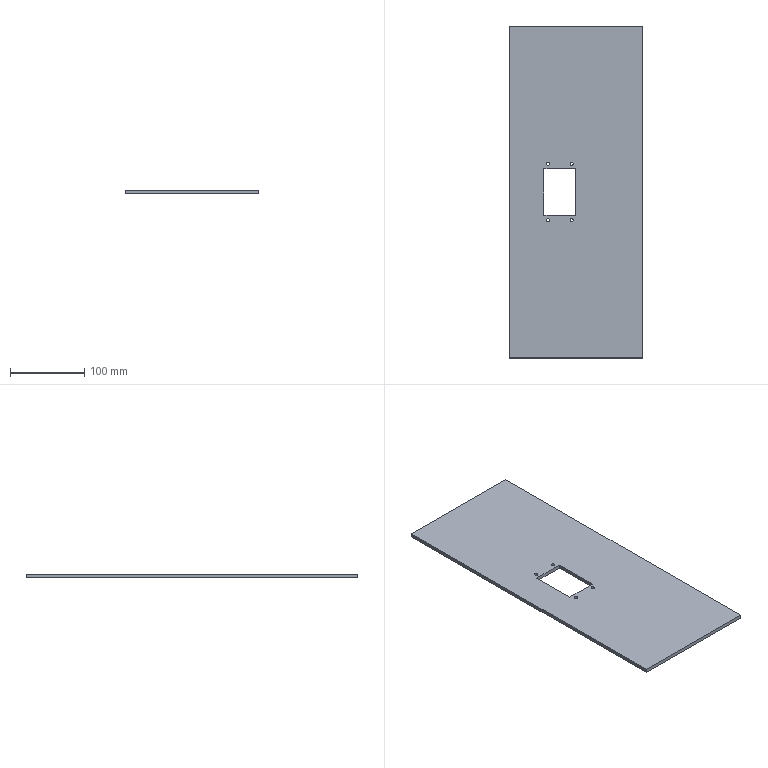Part | NX | features BREP 1 | 1 solid | 18 faces | box 179.5 x 447.9 x 5 mm | volume 388127 mm3 | plane 10 | cylinder 8 | commonest cylinder face diameters 4.5 x8
STEP:
#1=CARTESIAN_POINT('',(-8.,-38.,-2.5));
#2=VERTEX_POINT('',#1);
#3=CARTESIAN_POINT('',(-3.5,-38.,-2.5));
#4=VERTEX_POINT('',#3);
#5=CARTESIAN_POINT('',(-5.75,-38.,-2.5));
#6=DIRECTION('',(0.,0.,1.));
#7=DIRECTION('',(1.,0.,0.));
#8=AXIS2_PLACEMENT_3D('',#5,#6,#7);
#9=CIRCLE('',#8,2.25);
#10=EDGE_CURVE('',#2,#4,#9,.T.);
#11=ORIENTED_EDGE('',*,*,#10,.F.);
#12=CARTESIAN_POINT('',(-8.,-38.,2.5));
#13=VERTEX_POINT('',#12);
#14=CARTESIAN_POINT('',(-8.,-38.,-2.5));
#15=DIRECTION('',(0.,0.,1.));
#16=VECTOR('',#15,1000.);
#17=LINE('',#14,#16);
#18=EDGE_CURVE('',#13,#2,#17,.F.);
#19=ORIENTED_EDGE('',*,*,#18,.F.);
#20=CARTESIAN_POINT('',(-3.5,-38.,2.5));
#21=VERTEX_POINT('',#20);
#22=CARTESIAN_POINT('',(-5.75,-38.,2.5));
#23=DIRECTION('',(0.,0.,1.));
#24=DIRECTION('',(1.,0.,0.));
#25=AXIS2_PLACEMENT_3D('',#22,#23,#24);
#26=CIRCLE('',#25,2.25);
#27=EDGE_CURVE('',#13,#21,#26,.T.);
#28=ORIENTED_EDGE('',*,*,#27,.T.);
#29=CARTESIAN_POINT('',(-3.5,-38.,-2.5));
#30=DIRECTION('',(0.,0.,1.));
#31=VECTOR('',#30,1000.);
#32=LINE('',#29,#31);
#33=EDGE_CURVE('',#21,#4,#32,.F.);
#34=ORIENTED_EDGE('',*,*,#33,.T.);
#35=EDGE_LOOP('',(#11,#19,#28,#34));
#36=FACE_BOUND('',#35,.T.);
#37=CARTESIAN_POINT('',(-5.75,-38.,-2.5));
#38=DIRECTION('',(0.,0.,1.));
#39=DIRECTION('',(1.,0.,0.));
#40=AXIS2_PLACEMENT_3D('',#37,#38,#39);
#41=CYLINDRICAL_SURFACE('',#40,2.25);
#42=ADVANCED_FACE('',(#36),#41,.F.);
#43=CARTESIAN_POINT('',(-40.,-38.,-2.5));
#44=VERTEX_POINT('',#43);
#45=CARTESIAN_POINT('',(-35.5,-38.,-2.5));
#46=VERTEX_POINT('',#45);
#47=CARTESIAN_POINT('',(-37.75,-38.,-2.5));
#48=DIRECTION('',(0.,0.,1.));
#49=DIRECTION('',(1.,0.,0.));
#50=AXIS2_PLACEMENT_3D('',#47,#48,#49);
#51=CIRCLE('',#50,2.25);
#52=EDGE_CURVE('',#44,#46,#51,.T.);
#53=ORIENTED_EDGE('',*,*,#52,.F.);
#54=CARTESIAN_POINT('',(-40.,-38.,2.5));
#55=VERTEX_POINT('',#54);
#56=CARTESIAN_POINT('',(-40.,-38.,-2.5));
#57=DIRECTION('',(0.,0.,1.));
#58=VECTOR('',#57,1000.);
#59=LINE('',#56,#58);
#60=EDGE_CURVE('',#55,#44,#59,.F.);
#61=ORIENTED_EDGE('',*,*,#60,.F.);
#62=CARTESIAN_POINT('',(-35.5,-38.,2.5));
#63=VERTEX_POINT('',#62);
#64=CARTESIAN_POINT('',(-37.75,-38.,2.5));
#65=DIRECTION('',(0.,0.,1.));
#66=DIRECTION('',(1.,0.,0.));
#67=AXIS2_PLACEMENT_3D('',#64,#65,#66);
#68=CIRCLE('',#67,2.25);
#69=EDGE_CURVE('',#55,#63,#68,.T.);
#70=ORIENTED_EDGE('',*,*,#69,.T.);
#71=CARTESIAN_POINT('',(-35.5,-38.,-2.5));
#72=DIRECTION('',(0.,0.,1.));
#73=VECTOR('',#72,1000.);
#74=LINE('',#71,#73);
#75=EDGE_CURVE('',#63,#46,#74,.F.);
#76=ORIENTED_EDGE('',*,*,#75,.T.);
#77=EDGE_LOOP('',(#53,#61,#70,#76));
#78=FACE_BOUND('',#77,.T.);
#79=CARTESIAN_POINT('',(-37.75,-38.,-2.5));
#80=DIRECTION('',(0.,0.,1.));
#81=DIRECTION('',(1.,0.,0.));
#82=AXIS2_PLACEMENT_3D('',#79,#80,#81);
#83=CYLINDRICAL_SURFACE('',#82,2.25);
#84=ADVANCED_FACE('',(#78),#83,.F.);
#85=CARTESIAN_POINT('',(-8.,38.,-2.5));
#86=VERTEX_POINT('',#85);
#87=CARTESIAN_POINT('',(-3.5,38.,-2.5));
#88=VERTEX_POINT('',#87);
#89=CARTESIAN_POINT('',(-5.75,38.,-2.5));
#90=DIRECTION('',(0.,0.,1.));
#91=DIRECTION('',(1.,0.,0.));
#92=AXIS2_PLACEMENT_3D('',#89,#90,#91);
#93=CIRCLE('',#92,2.25);
#94=EDGE_CURVE('',#86,#88,#93,.T.);
#95=ORIENTED_EDGE('',*,*,#94,.F.);
#96=CARTESIAN_POINT('',(-8.,38.,2.5));
#97=VERTEX_POINT('',#96);
#98=CARTESIAN_POINT('',(-8.,38.,-2.5));
#99=DIRECTION('',(0.,0.,1.));
#100=VECTOR('',#99,1000.);
#101=LINE('',#98,#100);
#102=EDGE_CURVE('',#97,#86,#101,.F.);
#103=ORIENTED_EDGE('',*,*,#102,.F.);
#104=CARTESIAN_POINT('',(-3.5,38.,2.5));
#105=VERTEX_POINT('',#104);
#106=CARTESIAN_POINT('',(-5.75,38.,2.5));
#107=DIRECTION('',(0.,0.,1.));
#108=DIRECTION('',(1.,0.,0.));
#109=AXIS2_PLACEMENT_3D('',#106,#107,#108);
#110=CIRCLE('',#109,2.25);
#111=EDGE_CURVE('',#97,#105,#110,.T.);
#112=ORIENTED_EDGE('',*,*,#111,.T.);
#113=CARTESIAN_POINT('',(-3.5,38.,-2.5));
#114=DIRECTION('',(0.,0.,1.));
#115=VECTOR('',#114,1000.);
#116=LINE('',#113,#115);
#117=EDGE_CURVE('',#105,#88,#116,.F.);
#118=ORIENTED_EDGE('',*,*,#117,.T.);
#119=EDGE_LOOP('',(#95,#103,#112,#118));
#120=FACE_BOUND('',#119,.T.);
#121=CARTESIAN_POINT('',(-5.75,38.,-2.5));
#122=DIRECTION('',(0.,0.,1.));
#123=DIRECTION('',(1.,0.,0.));
#124=AXIS2_PLACEMENT_3D('',#121,#122,#123);
#125=CYLINDRICAL_SURFACE('',#124,2.25);
#126=ADVANCED_FACE('',(#120),#125,.F.);
#127=CARTESIAN_POINT('',(-40.,38.,-2.5));
#128=VERTEX_POINT('',#127);
#129=CARTESIAN_POINT('',(-35.5,38.,-2.5));
#130=VERTEX_POINT('',#129);
#131=CARTESIAN_POINT('',(-37.75,38.,-2.5));
#132=DIRECTION('',(0.,0.,1.));
#133=DIRECTION('',(1.,0.,0.));
#134=AXIS2_PLACEMENT_3D('',#131,#132,#133);
#135=CIRCLE('',#134,2.25);
#136=EDGE_CURVE('',#128,#130,#135,.T.);
#137=ORIENTED_EDGE('',*,*,#136,.F.);
#138=CARTESIAN_POINT('',(-40.,38.,2.5));
#139=VERTEX_POINT('',#138);
#140=CARTESIAN_POINT('',(-40.,38.,-2.5));
#141=DIRECTION('',(0.,0.,1.));
#142=VECTOR('',#141,1000.);
#143=LINE('',#140,#142);
#144=EDGE_CURVE('',#139,#128,#143,.F.);
#145=ORIENTED_EDGE('',*,*,#144,.F.);
#146=CARTESIAN_POINT('',(-35.5,38.,2.5));
#147=VERTEX_POINT('',#146);
#148=CARTESIAN_POINT('',(-37.75,38.,2.5));
#149=DIRECTION('',(0.,0.,1.));
#150=DIRECTION('',(1.,0.,0.));
#151=AXIS2_PLACEMENT_3D('',#148,#149,#150);
#152=CIRCLE('',#151,2.25);
#153=EDGE_CURVE('',#139,#147,#152,.T.);
#154=ORIENTED_EDGE('',*,*,#153,.T.);
#155=CARTESIAN_POINT('',(-35.5,38.,-2.5));
#156=DIRECTION('',(0.,0.,1.));
#157=VECTOR('',#156,1000.);
#158=LINE('',#155,#157);
#159=EDGE_CURVE('',#147,#130,#158,.F.);
#160=ORIENTED_EDGE('',*,*,#159,.T.);
#161=EDGE_LOOP('',(#137,#145,#154,#160));
#162=FACE_BOUND('',#161,.T.);
#163=CARTESIAN_POINT('',(-37.75,38.,-2.5));
#164=DIRECTION('',(0.,0.,1.));
#165=DIRECTION('',(1.,0.,0.));
#166=AXIS2_PLACEMENT_3D('',#163,#164,#165);
#167=CYLINDRICAL_SURFACE('',#166,2.25);
#168=ADVANCED_FACE('',(#162),#167,.F.);
#169=CARTESIAN_POINT('',(89.75,-223.95,-2.5));
#170=VERTEX_POINT('',#169);
#171=CARTESIAN_POINT('',(89.75,223.95,-2.5));
#172=VERTEX_POINT('',#171);
#173=CARTESIAN_POINT('',(89.75,-223.95,-2.5));
#174=DIRECTION('',(0.,1.,0.));
#175=VECTOR('',#174,1000.);
#176=LINE('',#173,#175);
#177=EDGE_CURVE('',#170,#172,#176,.T.);
#178=ORIENTED_EDGE('',*,*,#177,.T.);
#179=CARTESIAN_POINT('',(89.75,223.95,2.5));
#180=VERTEX_POINT('',#179);
#181=CARTESIAN_POINT('',(89.75,223.95,2.5));
#182=DIRECTION('',(0.,0.,-1.));
#183=VECTOR('',#182,1000.);
#184=LINE('',#181,#183);
#185=EDGE_CURVE('',#180,#172,#184,.T.);
#186=ORIENTED_EDGE('',*,*,#185,.F.);
#187=CARTESIAN_POINT('',(89.75,-223.95,2.5));
#188=VERTEX_POINT('',#187);
#189=CARTESIAN_POINT('',(89.75,-223.95,2.5));
#190=DIRECTION('',(0.,1.,0.));
#191=VECTOR('',#190,1000.);
#192=LINE('',#189,#191);
#193=EDGE_CURVE('',#188,#180,#192,.T.);
#194=ORIENTED_EDGE('',*,*,#193,.F.);
#195=CARTESIAN_POINT('',(89.75,-223.95,2.5));
#196=DIRECTION('',(0.,0.,-1.));
#197=VECTOR('',#196,1000.);
#198=LINE('',#195,#197);
#199=EDGE_CURVE('',#188,#170,#198,.T.);
#200=ORIENTED_EDGE('',*,*,#199,.T.);
#201=EDGE_LOOP('',(#178,#186,#194,#200));
#202=FACE_BOUND('',#201,.T.);
#203=CARTESIAN_POINT('',(89.75,-223.95,2.5));
#204=DIRECTION('',(-1.,0.,0.));
#205=DIRECTION('',(0.,0.,1.));
#206=AXIS2_PLACEMENT_3D('',#203,#204,#205);
#207=PLANE('',#206);
#208=ADVANCED_FACE('',(#202),#207,.F.);
#209=CARTESIAN_POINT('',(-89.75,223.95,-2.5));
#210=VERTEX_POINT('',#209);
#211=CARTESIAN_POINT('',(-89.75,223.95,-2.5));
#212=DIRECTION('',(-1.,0.,0.));
#213=VECTOR('',#212,1000.);
#214=LINE('',#211,#213);
#215=EDGE_CURVE('',#172,#210,#214,.T.);
#216=ORIENTED_EDGE('',*,*,#215,.T.);
#217=CARTESIAN_POINT('',(-89.75,223.95,2.5));
#218=VERTEX_POINT('',#217);
#219=CARTESIAN_POINT('',(-89.75,223.95,2.5));
#220=DIRECTION('',(0.,0.,-1.));
#221=VECTOR('',#220,1000.);
#222=LINE('',#219,#221);
#223=EDGE_CURVE('',#218,#210,#222,.T.);
#224=ORIENTED_EDGE('',*,*,#223,.F.);
#225=CARTESIAN_POINT('',(-89.75,223.95,2.5));
#226=DIRECTION('',(-1.,0.,0.));
#227=VECTOR('',#226,1000.);
#228=LINE('',#225,#227);
#229=EDGE_CURVE('',#180,#218,#228,.T.);
#230=ORIENTED_EDGE('',*,*,#229,.F.);
#231=ORIENTED_EDGE('',*,*,#185,.T.);
#232=EDGE_LOOP('',(#216,#224,#230,#231));
#233=FACE_BOUND('',#232,.T.);
#234=CARTESIAN_POINT('',(-89.75,223.95,2.5));
#235=DIRECTION('',(0.,-1.,0.));
#236=DIRECTION('',(0.,0.,-1.));
#237=AXIS2_PLACEMENT_3D('',#234,#235,#236);
#238=PLANE('',#237);
#239=ADVANCED_FACE('',(#233),#238,.F.);
#240=CARTESIAN_POINT('',(-89.75,-223.95,-2.5));
#241=VERTEX_POINT('',#240);
#242=CARTESIAN_POINT('',(-89.75,-223.95,-2.5));
#243=DIRECTION('',(0.,-1.,0.));
#244=VECTOR('',#243,1000.);
#245=LINE('',#242,#244);
#246=EDGE_CURVE('',#210,#241,#245,.T.);
#247=ORIENTED_EDGE('',*,*,#246,.T.);
#248=CARTESIAN_POINT('',(-89.75,-223.95,2.5));
#249=VERTEX_POINT('',#248);
#250=CARTESIAN_POINT('',(-89.75,-223.95,2.5));
#251=DIRECTION('',(0.,0.,-1.));
#252=VECTOR('',#251,1000.);
#253=LINE('',#250,#252);
#254=EDGE_CURVE('',#249,#241,#253,.T.);
#255=ORIENTED_EDGE('',*,*,#254,.F.);
#256=CARTESIAN_POINT('',(-89.75,-223.95,2.5));
#257=DIRECTION('',(0.,-1.,0.));
#258=VECTOR('',#257,1000.);
#259=LINE('',#256,#258);
#260=EDGE_CURVE('',#218,#249,#259,.T.);
#261=ORIENTED_EDGE('',*,*,#260,.F.);
#262=ORIENTED_EDGE('',*,*,#223,.T.);
#263=EDGE_LOOP('',(#247,#255,#261,#262));
#264=FACE_BOUND('',#263,.T.);
#265=CARTESIAN_POINT('',(-89.75,-223.95,2.5));
#266=DIRECTION('',(1.,0.,0.));
#267=DIRECTION('',(0.,1.,0.));
#268=AXIS2_PLACEMENT_3D('',#265,#266,#267);
#269=PLANE('',#268);
#270=ADVANCED_FACE('',(#264),#269,.F.);
#271=CARTESIAN_POINT('',(-89.75,-223.95,-2.5));
#272=DIRECTION('',(1.,0.,0.));
#273=VECTOR('',#272,1000.);
#274=LINE('',#271,#273);
#275=EDGE_CURVE('',#241,#170,#274,.T.);
#276=ORIENTED_EDGE('',*,*,#275,.T.);
#277=ORIENTED_EDGE('',*,*,#199,.F.);
#278=CARTESIAN_POINT('',(-89.75,-223.95,2.5));
#279=DIRECTION('',(1.,0.,0.));
#280=VECTOR('',#279,1000.);
#281=LINE('',#278,#280);
#282=EDGE_CURVE('',#249,#188,#281,.T.);
#283=ORIENTED_EDGE('',*,*,#282,.F.);
#284=ORIENTED_EDGE('',*,*,#254,.T.);
#285=EDGE_LOOP('',(#276,#277,#283,#284));
#286=FACE_BOUND('',#285,.T.);
#287=CARTESIAN_POINT('',(-89.75,-223.95,2.5));
#288=DIRECTION('',(0.,1.,0.));
#289=DIRECTION('',(1.,0.,0.));
#290=AXIS2_PLACEMENT_3D('',#287,#288,#289);
#291=PLANE('',#290);
#292=ADVANCED_FACE('',(#286),#291,.F.);
#293=ORIENTED_EDGE('',*,*,#193,.T.);
#294=ORIENTED_EDGE('',*,*,#229,.T.);
#295=ORIENTED_EDGE('',*,*,#260,.T.);
#296=ORIENTED_EDGE('',*,*,#282,.T.);
#297=EDGE_LOOP('',(#293,#294,#295,#296));
#298=FACE_BOUND('',#297,.T.);
#299=CARTESIAN_POINT('',(-5.75,-38.,2.5));
#300=DIRECTION('',(0.,0.,1.));
#301=DIRECTION('',(1.,0.,0.));
#302=AXIS2_PLACEMENT_3D('',#299,#300,#301);
#303=CIRCLE('',#302,2.25);
#304=EDGE_CURVE('',#21,#13,#303,.T.);
#305=ORIENTED_EDGE('',*,*,#304,.F.);
#306=ORIENTED_EDGE('',*,*,#27,.F.);
#307=EDGE_LOOP('',(#305,#306));
#308=FACE_BOUND('',#307,.T.);
#309=CARTESIAN_POINT('',(-37.75,-38.,2.5));
#310=DIRECTION('',(0.,0.,1.));
#311=DIRECTION('',(1.,0.,0.));
#312=AXIS2_PLACEMENT_3D('',#309,#310,#311);
#313=CIRCLE('',#312,2.25);
#314=EDGE_CURVE('',#63,#55,#313,.T.);
#315=ORIENTED_EDGE('',*,*,#314,.F.);
#316=ORIENTED_EDGE('',*,*,#69,.F.);
#317=EDGE_LOOP('',(#315,#316));
#318=FACE_BOUND('',#317,.T.);
#319=CARTESIAN_POINT('',(-5.75,38.,2.5));
#320=DIRECTION('',(0.,0.,1.));
#321=DIRECTION('',(1.,0.,0.));
#322=AXIS2_PLACEMENT_3D('',#319,#320,#321);
#323=CIRCLE('',#322,2.25);
#324=EDGE_CURVE('',#105,#97,#323,.T.);
#325=ORIENTED_EDGE('',*,*,#324,.F.);
#326=ORIENTED_EDGE('',*,*,#111,.F.);
#327=EDGE_LOOP('',(#325,#326));
#328=FACE_BOUND('',#327,.T.);
#329=CARTESIAN_POINT('',(-37.75,38.,2.5));
#330=DIRECTION('',(0.,0.,1.));
#331=DIRECTION('',(1.,0.,0.));
#332=AXIS2_PLACEMENT_3D('',#329,#330,#331);
#333=CIRCLE('',#332,2.25);
#334=EDGE_CURVE('',#147,#139,#333,.T.);
#335=ORIENTED_EDGE('',*,*,#334,.F.);
#336=ORIENTED_EDGE('',*,*,#153,.F.);
#337=EDGE_LOOP('',(#335,#336));
#338=FACE_BOUND('',#337,.T.);
#339=CARTESIAN_POINT('',(-0.25,31.5,2.5));
#340=VERTEX_POINT('',#339);
#341=CARTESIAN_POINT('',(-43.25,31.5,2.5));
#342=VERTEX_POINT('',#341);
#343=CARTESIAN_POINT('',(-43.25,31.5,2.5));
#344=DIRECTION('',(-1.,0.,0.));
#345=VECTOR('',#344,1000.);
#346=LINE('',#343,#345);
#347=EDGE_CURVE('',#340,#342,#346,.T.);
#348=ORIENTED_EDGE('',*,*,#347,.F.);
#349=CARTESIAN_POINT('',(-0.25,-31.5,2.5));
#350=VERTEX_POINT('',#349);
#351=CARTESIAN_POINT('',(-0.25,-31.5,2.5));
#352=DIRECTION('',(0.,1.,0.));
#353=VECTOR('',#352,1000.);
#354=LINE('',#351,#353);
#355=EDGE_CURVE('',#350,#340,#354,.T.);
#356=ORIENTED_EDGE('',*,*,#355,.F.);
#357=CARTESIAN_POINT('',(-43.25,-31.5,2.5));
#358=VERTEX_POINT('',#357);
#359=CARTESIAN_POINT('',(-43.25,-31.5,2.5));
#360=DIRECTION('',(1.,0.,0.));
#361=VECTOR('',#360,1000.);
#362=LINE('',#359,#361);
#363=EDGE_CURVE('',#358,#350,#362,.T.);
#364=ORIENTED_EDGE('',*,*,#363,.F.);
#365=CARTESIAN_POINT('',(-43.25,-31.5,2.5));
#366=DIRECTION('',(0.,-1.,0.));
#367=VECTOR('',#366,1000.);
#368=LINE('',#365,#367);
#369=EDGE_CURVE('',#342,#358,#368,.T.);
#370=ORIENTED_EDGE('',*,*,#369,.F.);
#371=EDGE_LOOP('',(#348,#356,#364,#370));
#372=FACE_BOUND('',#371,.T.);
#373=CARTESIAN_POINT('',(0.,0.,2.5));
#374=DIRECTION('',(0.,0.,-1.));
#375=DIRECTION('',(0.,-1.,0.));
#376=AXIS2_PLACEMENT_3D('',#373,#374,#375);
#377=PLANE('',#376);
#378=ADVANCED_FACE('',(#298,#308,#318,#328,#338,#372),#377,.F.);
#379=ORIENTED_EDGE('',*,*,#177,.F.);
#380=ORIENTED_EDGE('',*,*,#275,.F.);
#381=ORIENTED_EDGE('',*,*,#246,.F.);
#382=ORIENTED_EDGE('',*,*,#215,.F.);
#383=EDGE_LOOP('',(#379,#380,#381,#382));
#384=FACE_BOUND('',#383,.T.);
#385=CARTESIAN_POINT('',(-5.75,-38.,-2.5));
#386=DIRECTION('',(0.,0.,1.));
#387=DIRECTION('',(1.,0.,0.));
#388=AXIS2_PLACEMENT_3D('',#385,#386,#387);
#389=CIRCLE('',#388,2.25);
#390=EDGE_CURVE('',#4,#2,#389,.T.);
#391=ORIENTED_EDGE('',*,*,#390,.T.);
#392=ORIENTED_EDGE('',*,*,#10,.T.);
#393=EDGE_LOOP('',(#391,#392));
#394=FACE_BOUND('',#393,.T.);
#395=CARTESIAN_POINT('',(-37.75,-38.,-2.5));
#396=DIRECTION('',(0.,0.,1.));
#397=DIRECTION('',(1.,0.,0.));
#398=AXIS2_PLACEMENT_3D('',#395,#396,#397);
#399=CIRCLE('',#398,2.25);
#400=EDGE_CURVE('',#46,#44,#399,.T.);
#401=ORIENTED_EDGE('',*,*,#400,.T.);
#402=ORIENTED_EDGE('',*,*,#52,.T.);
#403=EDGE_LOOP('',(#401,#402));
#404=FACE_BOUND('',#403,.T.);
#405=CARTESIAN_POINT('',(-5.75,38.,-2.5));
#406=DIRECTION('',(0.,0.,1.));
#407=DIRECTION('',(1.,0.,0.));
#408=AXIS2_PLACEMENT_3D('',#405,#406,#407);
#409=CIRCLE('',#408,2.25);
#410=EDGE_CURVE('',#88,#86,#409,.T.);
#411=ORIENTED_EDGE('',*,*,#410,.T.);
#412=ORIENTED_EDGE('',*,*,#94,.T.);
#413=EDGE_LOOP('',(#411,#412));
#414=FACE_BOUND('',#413,.T.);
#415=CARTESIAN_POINT('',(-37.75,38.,-2.5));
#416=DIRECTION('',(0.,0.,1.));
#417=DIRECTION('',(1.,0.,0.));
#418=AXIS2_PLACEMENT_3D('',#415,#416,#417);
#419=CIRCLE('',#418,2.25);
#420=EDGE_CURVE('',#130,#128,#419,.T.);
#421=ORIENTED_EDGE('',*,*,#420,.T.);
#422=ORIENTED_EDGE('',*,*,#136,.T.);
#423=EDGE_LOOP('',(#421,#422));
#424=FACE_BOUND('',#423,.T.);
#425=CARTESIAN_POINT('',(-0.25,-31.5,-2.5));
#426=VERTEX_POINT('',#425);
#427=CARTESIAN_POINT('',(-0.25,31.5,-2.5));
#428=VERTEX_POINT('',#427);
#429=CARTESIAN_POINT('',(-0.25,-31.5,-2.5));
#430=DIRECTION('',(0.,1.,0.));
#431=VECTOR('',#430,1000.);
#432=LINE('',#429,#431);
#433=EDGE_CURVE('',#426,#428,#432,.T.);
#434=ORIENTED_EDGE('',*,*,#433,.T.);
#435=CARTESIAN_POINT('',(-43.25,31.5,-2.5));
#436=VERTEX_POINT('',#435);
#437=CARTESIAN_POINT('',(-43.25,31.5,-2.5));
#438=DIRECTION('',(-1.,0.,0.));
#439=VECTOR('',#438,1000.);
#440=LINE('',#437,#439);
#441=EDGE_CURVE('',#428,#436,#440,.T.);
#442=ORIENTED_EDGE('',*,*,#441,.T.);
#443=CARTESIAN_POINT('',(-43.25,-31.5,-2.5));
#444=VERTEX_POINT('',#443);
#445=CARTESIAN_POINT('',(-43.25,-31.5,-2.5));
#446=DIRECTION('',(0.,-1.,0.));
#447=VECTOR('',#446,1000.);
#448=LINE('',#445,#447);
#449=EDGE_CURVE('',#436,#444,#448,.T.);
#450=ORIENTED_EDGE('',*,*,#449,.T.);
#451=CARTESIAN_POINT('',(-43.25,-31.5,-2.5));
#452=DIRECTION('',(1.,0.,0.));
#453=VECTOR('',#452,1000.);
#454=LINE('',#451,#453);
#455=EDGE_CURVE('',#444,#426,#454,.T.);
#456=ORIENTED_EDGE('',*,*,#455,.T.);
#457=EDGE_LOOP('',(#434,#442,#450,#456));
#458=FACE_BOUND('',#457,.T.);
#459=CARTESIAN_POINT('',(0.,0.,-2.5));
#460=DIRECTION('',(0.,0.,-1.));
#461=DIRECTION('',(0.,-1.,0.));
#462=AXIS2_PLACEMENT_3D('',#459,#460,#461);
#463=PLANE('',#462);
#464=ADVANCED_FACE('',(#384,#394,#404,#414,#424,#458),#463,.T.);
#465=CARTESIAN_POINT('',(-0.25,31.5,-2.5));
#466=DIRECTION('',(0.,0.,1.));
#467=VECTOR('',#466,1000.);
#468=LINE('',#465,#467);
#469=EDGE_CURVE('',#428,#340,#468,.T.);
#470=ORIENTED_EDGE('',*,*,#469,.F.);
#471=ORIENTED_EDGE('',*,*,#433,.F.);
#472=CARTESIAN_POINT('',(-0.25,-31.5,-2.5));
#473=DIRECTION('',(0.,0.,1.));
#474=VECTOR('',#473,1000.);
#475=LINE('',#472,#474);
#476=EDGE_CURVE('',#426,#350,#475,.T.);
#477=ORIENTED_EDGE('',*,*,#476,.T.);
#478=ORIENTED_EDGE('',*,*,#355,.T.);
#479=EDGE_LOOP('',(#470,#471,#477,#478));
#480=FACE_BOUND('',#479,.T.);
#481=CARTESIAN_POINT('',(-0.25,-31.5,-2.5));
#482=DIRECTION('',(1.,0.,0.));
#483=DIRECTION('',(0.,1.,0.));
#484=AXIS2_PLACEMENT_3D('',#481,#482,#483);
#485=PLANE('',#484);
#486=ADVANCED_FACE('',(#480),#485,.F.);
#487=ORIENTED_EDGE('',*,*,#476,.F.);
#488=ORIENTED_EDGE('',*,*,#455,.F.);
#489=CARTESIAN_POINT('',(-43.25,-31.5,-2.5));
#490=DIRECTION('',(0.,0.,1.));
#491=VECTOR('',#490,1000.);
#492=LINE('',#489,#491);
#493=EDGE_CURVE('',#444,#358,#492,.T.);
#494=ORIENTED_EDGE('',*,*,#493,.T.);
#495=ORIENTED_EDGE('',*,*,#363,.T.);
#496=EDGE_LOOP('',(#487,#488,#494,#495));
#497=FACE_BOUND('',#496,.T.);
#498=CARTESIAN_POINT('',(-43.25,-31.5,-2.5));
#499=DIRECTION('',(0.,-1.,0.));
#500=DIRECTION('',(0.,0.,-1.));
#501=AXIS2_PLACEMENT_3D('',#498,#499,#500);
#502=PLANE('',#501);
#503=ADVANCED_FACE('',(#497),#502,.F.);
#504=ORIENTED_EDGE('',*,*,#493,.F.);
#505=ORIENTED_EDGE('',*,*,#449,.F.);
#506=CARTESIAN_POINT('',(-43.25,31.5,-2.5));
#507=DIRECTION('',(0.,0.,1.));
#508=VECTOR('',#507,1000.);
#509=LINE('',#506,#508);
#510=EDGE_CURVE('',#436,#342,#509,.T.);
#511=ORIENTED_EDGE('',*,*,#510,.T.);
#512=ORIENTED_EDGE('',*,*,#369,.T.);
#513=EDGE_LOOP('',(#504,#505,#511,#512));
#514=FACE_BOUND('',#513,.T.);
#515=CARTESIAN_POINT('',(-43.25,-31.5,-2.5));
#516=DIRECTION('',(-1.,0.,0.));
#517=DIRECTION('',(0.,0.,1.));
#518=AXIS2_PLACEMENT_3D('',#515,#516,#517);
#519=PLANE('',#518);
#520=ADVANCED_FACE('',(#514),#519,.F.);
#521=ORIENTED_EDGE('',*,*,#510,.F.);
#522=ORIENTED_EDGE('',*,*,#441,.F.);
#523=ORIENTED_EDGE('',*,*,#469,.T.);
#524=ORIENTED_EDGE('',*,*,#347,.T.);
#525=EDGE_LOOP('',(#521,#522,#523,#524));
#526=FACE_BOUND('',#525,.T.);
#527=CARTESIAN_POINT('',(-43.25,31.5,-2.5));
#528=DIRECTION('',(0.,1.,0.));
#529=DIRECTION('',(1.,0.,0.));
#530=AXIS2_PLACEMENT_3D('',#527,#528,#529);
#531=PLANE('',#530);
#532=ADVANCED_FACE('',(#526),#531,.F.);
#533=ORIENTED_EDGE('',*,*,#144,.T.);
#534=ORIENTED_EDGE('',*,*,#420,.F.);
#535=ORIENTED_EDGE('',*,*,#159,.F.);
#536=ORIENTED_EDGE('',*,*,#334,.T.);
#537=EDGE_LOOP('',(#533,#534,#535,#536));
#538=FACE_BOUND('',#537,.T.);
#539=CARTESIAN_POINT('',(-37.75,38.,-2.5));
#540=DIRECTION('',(0.,0.,1.));
#541=DIRECTION('',(1.,0.,0.));
#542=AXIS2_PLACEMENT_3D('',#539,#540,#541);
#543=CYLINDRICAL_SURFACE('',#542,2.25);
#544=ADVANCED_FACE('',(#538),#543,.F.);
#545=ORIENTED_EDGE('',*,*,#102,.T.);
#546=ORIENTED_EDGE('',*,*,#410,.F.);
#547=ORIENTED_EDGE('',*,*,#117,.F.);
#548=ORIENTED_EDGE('',*,*,#324,.T.);
#549=EDGE_LOOP('',(#545,#546,#547,#548));
#550=FACE_BOUND('',#549,.T.);
#551=CARTESIAN_POINT('',(-5.75,38.,-2.5));
#552=DIRECTION('',(0.,0.,1.));
#553=DIRECTION('',(1.,0.,0.));
#554=AXIS2_PLACEMENT_3D('',#551,#552,#553);
#555=CYLINDRICAL_SURFACE('',#554,2.25);
#556=ADVANCED_FACE('',(#550),#555,.F.);
#557=ORIENTED_EDGE('',*,*,#60,.T.);
#558=ORIENTED_EDGE('',*,*,#400,.F.);
#559=ORIENTED_EDGE('',*,*,#75,.F.);
#560=ORIENTED_EDGE('',*,*,#314,.T.);
#561=EDGE_LOOP('',(#557,#558,#559,#560));
#562=FACE_BOUND('',#561,.T.);
#563=CARTESIAN_POINT('',(-37.75,-38.,-2.5));
#564=DIRECTION('',(0.,0.,1.));
#565=DIRECTION('',(1.,0.,0.));
#566=AXIS2_PLACEMENT_3D('',#563,#564,#565);
#567=CYLINDRICAL_SURFACE('',#566,2.25);
#568=ADVANCED_FACE('',(#562),#567,.F.);
#569=ORIENTED_EDGE('',*,*,#18,.T.);
#570=ORIENTED_EDGE('',*,*,#390,.F.);
#571=ORIENTED_EDGE('',*,*,#33,.F.);
#572=ORIENTED_EDGE('',*,*,#304,.T.);
#573=EDGE_LOOP('',(#569,#570,#571,#572));
#574=FACE_BOUND('',#573,.T.);
#575=CARTESIAN_POINT('',(-5.75,-38.,-2.5));
#576=DIRECTION('',(0.,0.,1.));
#577=DIRECTION('',(1.,0.,0.));
#578=AXIS2_PLACEMENT_3D('',#575,#576,#577);
#579=CYLINDRICAL_SURFACE('',#578,2.25);
#580=ADVANCED_FACE('',(#574),#579,.F.);
#581=CLOSED_SHELL('',(#42,#84,#126,#168,#208,#239,#270,#292,#378,#464,#486,#503,#520,#532,#544,#556,#568,#580));
#582=MANIFOLD_SOLID_BREP('',#581);
#583=(LENGTH_UNIT()NAMED_UNIT(*)SI_UNIT(.MILLI.,.METRE.));
#584=UNCERTAINTY_MEASURE_WITH_UNIT(LENGTH_MEASURE(0.00001),#583,'','');
#585=(NAMED_UNIT(*)PLANE_ANGLE_UNIT()SI_UNIT($,.RADIAN.));
#586=(NAMED_UNIT(*)SI_UNIT($,.STERADIAN.)SOLID_ANGLE_UNIT());
#587=(GEOMETRIC_REPRESENTATION_CONTEXT(3)GLOBAL_UNCERTAINTY_ASSIGNED_CONTEXT((#584))GLOBAL_UNIT_ASSIGNED_CONTEXT((#583,#585,#586))REPRESENTATION_CONTEXT('',''));
#588=ADVANCED_BREP_SHAPE_REPRESENTATION('',(#582),#587);